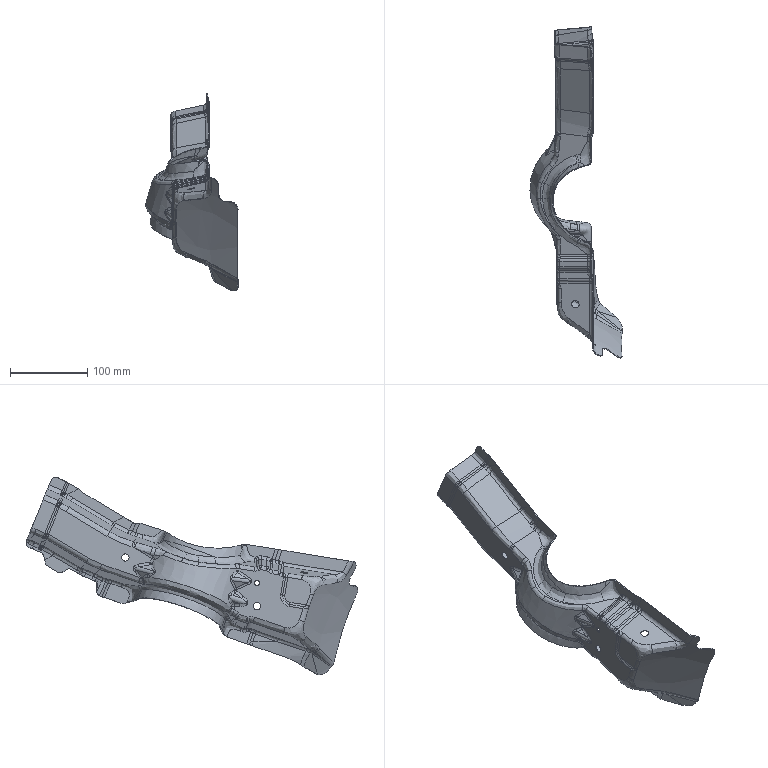Part | 1 solid | 735 faces | box 119.285 x 428.509 x 255.334 mm | volume 88742 mm3 | spline 523 | cylinder 138 | plane 58 | sphere 16 | commonest cylinder face diameters 10 x39 12.4 x28 12 x10 7.6 x9 9.6 x5 14.4 x5